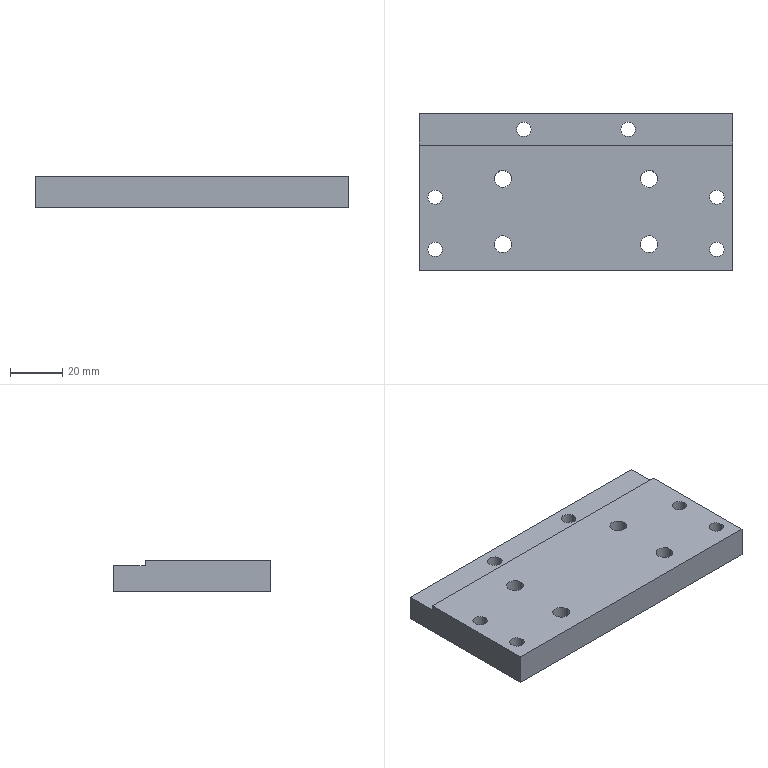Part | STEP file | 2042 Mounting base plate 3 | 1 solid | 46 faces | box 120 x 60 x 12 mm | volume 78438 mm3 | cylinder 32 | plane 14 | commonest cylinder face diameters 5.5 x12 10 x12 6.5 x8